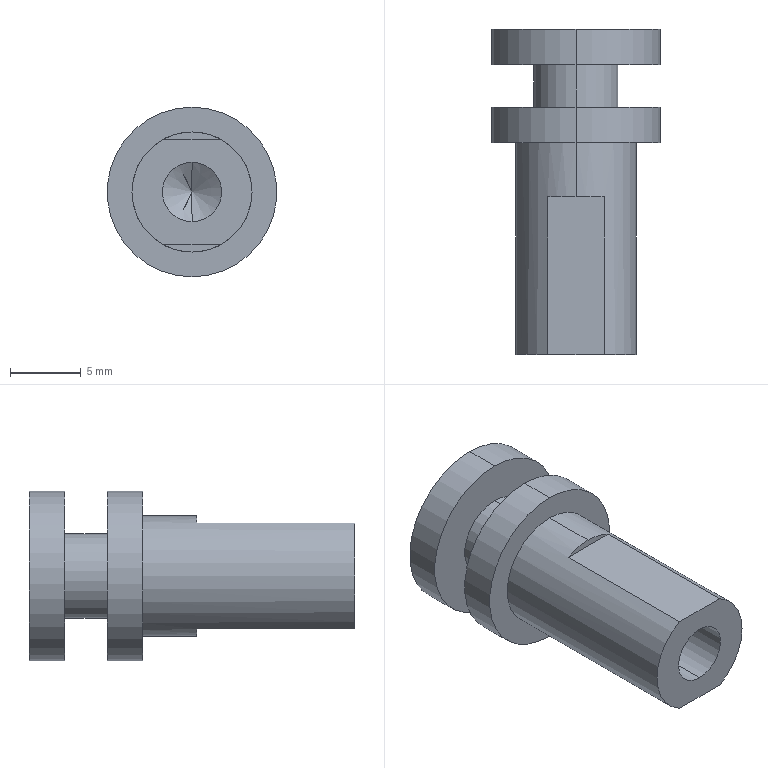Part | SolidWorks | features ICE 5, 3DProfileFeature 1, Extrusion 1, HoleWzd 1 | 1 solid | 21 faces | box 12 x 23 x 12 mm | volume 1299 mm3 | cylinder 10 | plane 9 | cone 2 | commonest cylinder face diameters 12 x4 4.2 x2 6 x2 8.5 x2
STEP:
#1=CARTESIAN_POINT('',(0.,-5.5,2.1));
#2=VERTEX_POINT('',#1);
#3=CARTESIAN_POINT('',(0.,-5.5,-2.1));
#4=VERTEX_POINT('',#3);
#5=CARTESIAN_POINT('',(0.,-5.5,0.));
#6=DIRECTION('',(0.,-1.,0.));
#7=DIRECTION('',(0.,0.,-1.));
#8=AXIS2_PLACEMENT_3D('',#5,#6,#7);
#9=CIRCLE('',#8,2.1);
#10=EDGE_CURVE('',#2,#4,#9,.T.);
#11=ORIENTED_EDGE('',*,*,#10,.F.);
#12=CARTESIAN_POINT('',(0.,-17.5,2.1));
#13=VERTEX_POINT('',#12);
#14=CARTESIAN_POINT('',(0.,-17.5,2.1));
#15=DIRECTION('',(0.,-1.,0.));
#16=VECTOR('',#15,1000.);
#17=LINE('',#14,#16);
#18=EDGE_CURVE('',#2,#13,#17,.T.);
#19=ORIENTED_EDGE('',*,*,#18,.T.);
#20=CARTESIAN_POINT('',(0.,-17.5,-2.1));
#21=VERTEX_POINT('',#20);
#22=CARTESIAN_POINT('',(0.,-17.5,0.));
#23=DIRECTION('',(0.,-1.,0.));
#24=DIRECTION('',(0.,0.,-1.));
#25=AXIS2_PLACEMENT_3D('',#22,#23,#24);
#26=CIRCLE('',#25,2.1);
#27=EDGE_CURVE('',#13,#21,#26,.T.);
#28=ORIENTED_EDGE('',*,*,#27,.T.);
#29=CARTESIAN_POINT('',(0.,-17.5,-2.1));
#30=DIRECTION('',(0.,-1.,0.));
#31=VECTOR('',#30,1000.);
#32=LINE('',#29,#31);
#33=EDGE_CURVE('',#4,#21,#32,.T.);
#34=ORIENTED_EDGE('',*,*,#33,.F.);
#35=EDGE_LOOP('',(#11,#19,#28,#34));
#36=FACE_OUTER_BOUND('',#35,.T.);
#37=CARTESIAN_POINT('',(0.,-17.5,0.));
#38=DIRECTION('',(0.,-1.,0.));
#39=DIRECTION('',(0.,0.,-1.));
#40=AXIS2_PLACEMENT_3D('',#37,#38,#39);
#41=CYLINDRICAL_SURFACE('',#40,2.1);
#42=ADVANCED_FACE('',(#36),#41,.F.);
#43=CARTESIAN_POINT('',(0.,-4.238,0.));
#44=VERTEX_POINT('',#43);
#45=CARTESIAN_POINT('',(0.,-5.5,-2.1));
#46=DIRECTION('',(0.,-0.515,-0.8572));
#47=VECTOR('',#46,1000.);
#48=LINE('',#45,#47);
#49=EDGE_CURVE('',#44,#4,#48,.T.);
#50=ORIENTED_EDGE('',*,*,#49,.F.);
#51=CARTESIAN_POINT('',(0.,-5.5,2.1));
#52=DIRECTION('',(0.,-0.515,0.8572));
#53=VECTOR('',#52,1000.);
#54=LINE('',#51,#53);
#55=EDGE_CURVE('',#44,#2,#54,.T.);
#56=ORIENTED_EDGE('',*,*,#55,.T.);
#57=ORIENTED_EDGE('',*,*,#10,.T.);
#58=EDGE_LOOP('',(#50,#56,#57));
#59=FACE_OUTER_BOUND('',#58,.T.);
#60=CARTESIAN_POINT('',(0.,-5.5,0.));
#61=DIRECTION('',(0.,-1.,0.));
#62=DIRECTION('',(0.,0.,-1.));
#63=AXIS2_PLACEMENT_3D('',#60,#61,#62);
#64=CONICAL_SURFACE('',#63,2.1,1.03);
#65=ADVANCED_FACE('',(#59),#64,.F.);
#66=CARTESIAN_POINT('',(2.,-6.347,-3.75));
#67=VERTEX_POINT('',#66);
#68=CARTESIAN_POINT('',(0.,-6.347,-4.25));
#69=VERTEX_POINT('',#68);
#70=CARTESIAN_POINT('',(0.,-6.347,0.));
#71=DIRECTION('',(0.,1.,0.));
#72=DIRECTION('',(0.,0.,1.));
#73=AXIS2_PLACEMENT_3D('',#70,#71,#72);
#74=CIRCLE('',#73,4.25);
#75=EDGE_CURVE('',#67,#69,#74,.T.);
#76=ORIENTED_EDGE('',*,*,#75,.T.);
#77=CARTESIAN_POINT('',(0.,-2.5,-4.25));
#78=VERTEX_POINT('',#77);
#79=CARTESIAN_POINT('',(0.,-17.5,-4.25));
#80=DIRECTION('',(0.,1.,0.));
#81=VECTOR('',#80,1000.);
#82=LINE('',#79,#81);
#83=EDGE_CURVE('',#69,#78,#82,.T.);
#84=ORIENTED_EDGE('',*,*,#83,.T.);
#85=CARTESIAN_POINT('',(0.,-2.5,4.25));
#86=VERTEX_POINT('',#85);
#87=CARTESIAN_POINT('',(0.,-2.5,0.));
#88=DIRECTION('',(0.,-1.,0.));
#89=DIRECTION('',(0.,0.,-1.));
#90=AXIS2_PLACEMENT_3D('',#87,#88,#89);
#91=CIRCLE('',#90,4.25);
#92=EDGE_CURVE('',#78,#86,#91,.T.);
#93=ORIENTED_EDGE('',*,*,#92,.T.);
#94=CARTESIAN_POINT('',(0.,-6.347,4.25));
#95=VERTEX_POINT('',#94);
#96=CARTESIAN_POINT('',(0.,-17.5,4.25));
#97=DIRECTION('',(0.,1.,0.));
#98=VECTOR('',#97,1000.);
#99=LINE('',#96,#98);
#100=EDGE_CURVE('',#95,#86,#99,.T.);
#101=ORIENTED_EDGE('',*,*,#100,.F.);
#102=CARTESIAN_POINT('',(2.,-6.347,3.75));
#103=VERTEX_POINT('',#102);
#104=CARTESIAN_POINT('',(0.,-6.347,0.));
#105=DIRECTION('',(0.,1.,0.));
#106=DIRECTION('',(0.,0.,1.));
#107=AXIS2_PLACEMENT_3D('',#104,#105,#106);
#108=CIRCLE('',#107,4.25);
#109=EDGE_CURVE('',#95,#103,#108,.T.);
#110=ORIENTED_EDGE('',*,*,#109,.T.);
#111=CARTESIAN_POINT('',(2.,-17.5,3.75));
#112=VERTEX_POINT('',#111);
#113=CARTESIAN_POINT('',(2.,-17.5,3.75));
#114=DIRECTION('',(0.,-1.,0.));
#115=VECTOR('',#114,1000.);
#116=LINE('',#113,#115);
#117=EDGE_CURVE('',#103,#112,#116,.T.);
#118=ORIENTED_EDGE('',*,*,#117,.T.);
#119=CARTESIAN_POINT('',(2.,-17.5,-3.75));
#120=VERTEX_POINT('',#119);
#121=CARTESIAN_POINT('',(0.,-17.5,0.));
#122=DIRECTION('',(0.,-1.,0.));
#123=DIRECTION('',(0.,0.,-1.));
#124=AXIS2_PLACEMENT_3D('',#121,#122,#123);
#125=CIRCLE('',#124,4.25);
#126=EDGE_CURVE('',#120,#112,#125,.T.);
#127=ORIENTED_EDGE('',*,*,#126,.F.);
#128=CARTESIAN_POINT('',(2.,-17.5,-3.75));
#129=DIRECTION('',(0.,1.,0.));
#130=VECTOR('',#129,1000.);
#131=LINE('',#128,#130);
#132=EDGE_CURVE('',#120,#67,#131,.T.);
#133=ORIENTED_EDGE('',*,*,#132,.T.);
#134=EDGE_LOOP('',(#76,#84,#93,#101,#110,#118,#127,#133));
#135=FACE_OUTER_BOUND('',#134,.T.);
#136=CARTESIAN_POINT('',(0.,-17.5,0.));
#137=DIRECTION('',(0.,1.,0.));
#138=DIRECTION('',(0.,0.,1.));
#139=AXIS2_PLACEMENT_3D('',#136,#137,#138);
#140=CYLINDRICAL_SURFACE('',#139,4.25);
#141=ADVANCED_FACE('',(#135),#140,.T.);
#142=CARTESIAN_POINT('',(0.,-2.5,-6.));
#143=VERTEX_POINT('',#142);
#144=CARTESIAN_POINT('',(0.,-2.5,6.));
#145=VERTEX_POINT('',#144);
#146=CARTESIAN_POINT('',(0.,-2.5,0.));
#147=DIRECTION('',(0.,-1.,0.));
#148=DIRECTION('',(0.,0.,-1.));
#149=AXIS2_PLACEMENT_3D('',#146,#147,#148);
#150=CIRCLE('',#149,6.);
#151=EDGE_CURVE('',#143,#145,#150,.T.);
#152=ORIENTED_EDGE('',*,*,#151,.F.);
#153=CARTESIAN_POINT('',(0.,0.,-6.));
#154=VERTEX_POINT('',#153);
#155=CARTESIAN_POINT('',(0.,-2.5,-6.));
#156=DIRECTION('',(0.,1.,0.));
#157=VECTOR('',#156,1000.);
#158=LINE('',#155,#157);
#159=EDGE_CURVE('',#143,#154,#158,.T.);
#160=ORIENTED_EDGE('',*,*,#159,.T.);
#161=CARTESIAN_POINT('',(0.,0.,6.));
#162=VERTEX_POINT('',#161);
#163=CARTESIAN_POINT('',(0.,0.,0.));
#164=DIRECTION('',(0.,-1.,0.));
#165=DIRECTION('',(0.,0.,-1.));
#166=AXIS2_PLACEMENT_3D('',#163,#164,#165);
#167=CIRCLE('',#166,6.);
#168=EDGE_CURVE('',#154,#162,#167,.T.);
#169=ORIENTED_EDGE('',*,*,#168,.T.);
#170=CARTESIAN_POINT('',(0.,-2.5,6.));
#171=DIRECTION('',(0.,1.,0.));
#172=VECTOR('',#171,1000.);
#173=LINE('',#170,#172);
#174=EDGE_CURVE('',#145,#162,#173,.T.);
#175=ORIENTED_EDGE('',*,*,#174,.F.);
#176=EDGE_LOOP('',(#152,#160,#169,#175));
#177=FACE_OUTER_BOUND('',#176,.T.);
#178=CARTESIAN_POINT('',(0.,-2.5,0.));
#179=DIRECTION('',(0.,1.,0.));
#180=DIRECTION('',(0.,0.,1.));
#181=AXIS2_PLACEMENT_3D('',#178,#179,#180);
#182=CYLINDRICAL_SURFACE('',#181,6.);
#183=ADVANCED_FACE('',(#177),#182,.T.);
#184=CARTESIAN_POINT('',(0.,5.5,6.));
#185=VERTEX_POINT('',#184);
#186=CARTESIAN_POINT('',(0.,5.5,-6.));
#187=VERTEX_POINT('',#186);
#188=CARTESIAN_POINT('',(0.,5.5,0.));
#189=DIRECTION('',(0.,1.,0.));
#190=DIRECTION('',(0.,0.,1.));
#191=AXIS2_PLACEMENT_3D('',#188,#189,#190);
#192=CIRCLE('',#191,6.);
#193=EDGE_CURVE('',#185,#187,#192,.T.);
#194=ORIENTED_EDGE('',*,*,#193,.F.);
#195=CARTESIAN_POINT('',(0.,3.,6.));
#196=VERTEX_POINT('',#195);
#197=CARTESIAN_POINT('',(0.,5.5,6.));
#198=DIRECTION('',(0.,-1.,0.));
#199=VECTOR('',#198,1000.);
#200=LINE('',#197,#199);
#201=EDGE_CURVE('',#185,#196,#200,.T.);
#202=ORIENTED_EDGE('',*,*,#201,.T.);
#203=CARTESIAN_POINT('',(0.,3.,-6.));
#204=VERTEX_POINT('',#203);
#205=CARTESIAN_POINT('',(0.,3.,0.));
#206=DIRECTION('',(0.,1.,0.));
#207=DIRECTION('',(0.,0.,1.));
#208=AXIS2_PLACEMENT_3D('',#205,#206,#207);
#209=CIRCLE('',#208,6.);
#210=EDGE_CURVE('',#196,#204,#209,.T.);
#211=ORIENTED_EDGE('',*,*,#210,.T.);
#212=CARTESIAN_POINT('',(0.,5.5,-6.));
#213=DIRECTION('',(0.,-1.,0.));
#214=VECTOR('',#213,1000.);
#215=LINE('',#212,#214);
#216=EDGE_CURVE('',#187,#204,#215,.T.);
#217=ORIENTED_EDGE('',*,*,#216,.F.);
#218=EDGE_LOOP('',(#194,#202,#211,#217));
#219=FACE_OUTER_BOUND('',#218,.T.);
#220=CARTESIAN_POINT('',(0.,5.5,0.));
#221=DIRECTION('',(0.,-1.,0.));
#222=DIRECTION('',(0.,0.,-1.));
#223=AXIS2_PLACEMENT_3D('',#220,#221,#222);
#224=CYLINDRICAL_SURFACE('',#223,6.);
#225=ADVANCED_FACE('',(#219),#224,.T.);
#226=CARTESIAN_POINT('',(0.,3.,3.));
#227=VERTEX_POINT('',#226);
#228=CARTESIAN_POINT('',(0.,3.,-3.));
#229=VERTEX_POINT('',#228);
#230=CARTESIAN_POINT('',(0.,3.,0.));
#231=DIRECTION('',(0.,1.,0.));
#232=DIRECTION('',(0.,0.,1.));
#233=AXIS2_PLACEMENT_3D('',#230,#231,#232);
#234=CIRCLE('',#233,3.);
#235=EDGE_CURVE('',#227,#229,#234,.T.);
#236=ORIENTED_EDGE('',*,*,#235,.F.);
#237=CARTESIAN_POINT('',(0.,0.,3.));
#238=VERTEX_POINT('',#237);
#239=CARTESIAN_POINT('',(0.,3.,3.));
#240=DIRECTION('',(0.,-1.,0.));
#241=VECTOR('',#240,1000.);
#242=LINE('',#239,#241);
#243=EDGE_CURVE('',#227,#238,#242,.T.);
#244=ORIENTED_EDGE('',*,*,#243,.T.);
#245=CARTESIAN_POINT('',(0.,0.,-3.));
#246=VERTEX_POINT('',#245);
#247=CARTESIAN_POINT('',(0.,0.,0.));
#248=DIRECTION('',(0.,-1.,0.));
#249=DIRECTION('',(0.,0.,-1.));
#250=AXIS2_PLACEMENT_3D('',#247,#248,#249);
#251=CIRCLE('',#250,3.);
#252=EDGE_CURVE('',#246,#238,#251,.T.);
#253=ORIENTED_EDGE('',*,*,#252,.F.);
#254=CARTESIAN_POINT('',(0.,3.,-3.));
#255=DIRECTION('',(0.,-1.,0.));
#256=VECTOR('',#255,1000.);
#257=LINE('',#254,#256);
#258=EDGE_CURVE('',#229,#246,#257,.T.);
#259=ORIENTED_EDGE('',*,*,#258,.F.);
#260=EDGE_LOOP('',(#236,#244,#253,#259));
#261=FACE_OUTER_BOUND('',#260,.T.);
#262=CARTESIAN_POINT('',(0.,3.,0.));
#263=DIRECTION('',(0.,-1.,0.));
#264=DIRECTION('',(0.,0.,-1.));
#265=AXIS2_PLACEMENT_3D('',#262,#263,#264);
#266=CYLINDRICAL_SURFACE('',#265,3.);
#267=ADVANCED_FACE('',(#261),#266,.T.);
#268=CARTESIAN_POINT('',(0.,-2.5,0.));
#269=DIRECTION('',(0.,-1.,0.));
#270=DIRECTION('',(0.,0.,-1.));
#271=AXIS2_PLACEMENT_3D('',#268,#269,#270);
#272=CIRCLE('',#271,6.);
#273=EDGE_CURVE('',#145,#143,#272,.T.);
#274=ORIENTED_EDGE('',*,*,#273,.T.);
#275=ORIENTED_EDGE('',*,*,#151,.T.);
#276=EDGE_LOOP('',(#274,#275));
#277=FACE_OUTER_BOUND('',#276,.T.);
#278=CARTESIAN_POINT('',(0.,-2.5,0.));
#279=DIRECTION('',(0.,-1.,0.));
#280=DIRECTION('',(0.,0.,-1.));
#281=AXIS2_PLACEMENT_3D('',#278,#279,#280);
#282=CIRCLE('',#281,4.25);
#283=EDGE_CURVE('',#86,#78,#282,.T.);
#284=ORIENTED_EDGE('',*,*,#283,.F.);
#285=ORIENTED_EDGE('',*,*,#92,.F.);
#286=EDGE_LOOP('',(#284,#285));
#287=FACE_BOUND('',#286,.T.);
#288=CARTESIAN_POINT('',(0.,-2.5,0.));
#289=DIRECTION('',(0.,-1.,0.));
#290=DIRECTION('',(0.,0.,-1.));
#291=AXIS2_PLACEMENT_3D('',#288,#289,#290);
#292=PLANE('',#291);
#293=ADVANCED_FACE('',(#277,#287),#292,.T.);
#294=ORIENTED_EDGE('',*,*,#243,.F.);
#295=CARTESIAN_POINT('',(0.,3.,0.));
#296=DIRECTION('',(0.,1.,0.));
#297=DIRECTION('',(0.,0.,1.));
#298=AXIS2_PLACEMENT_3D('',#295,#296,#297);
#299=CIRCLE('',#298,3.);
#300=EDGE_CURVE('',#229,#227,#299,.T.);
#301=ORIENTED_EDGE('',*,*,#300,.F.);
#302=ORIENTED_EDGE('',*,*,#258,.T.);
#303=CARTESIAN_POINT('',(0.,0.,0.));
#304=DIRECTION('',(0.,-1.,0.));
#305=DIRECTION('',(0.,0.,-1.));
#306=AXIS2_PLACEMENT_3D('',#303,#304,#305);
#307=CIRCLE('',#306,3.);
#308=EDGE_CURVE('',#238,#246,#307,.T.);
#309=ORIENTED_EDGE('',*,*,#308,.F.);
#310=EDGE_LOOP('',(#294,#301,#302,#309));
#311=FACE_OUTER_BOUND('',#310,.T.);
#312=CARTESIAN_POINT('',(0.,3.,0.));
#313=DIRECTION('',(0.,-1.,0.));
#314=DIRECTION('',(0.,0.,-1.));
#315=AXIS2_PLACEMENT_3D('',#312,#313,#314);
#316=CYLINDRICAL_SURFACE('',#315,3.);
#317=ADVANCED_FACE('',(#311),#316,.T.);
#318=CARTESIAN_POINT('',(0.,3.,0.));
#319=DIRECTION('',(0.,1.,0.));
#320=DIRECTION('',(0.,0.,1.));
#321=AXIS2_PLACEMENT_3D('',#318,#319,#320);
#322=CIRCLE('',#321,6.);
#323=EDGE_CURVE('',#204,#196,#322,.T.);
#324=ORIENTED_EDGE('',*,*,#323,.F.);
#325=ORIENTED_EDGE('',*,*,#210,.F.);
#326=EDGE_LOOP('',(#324,#325));
#327=FACE_OUTER_BOUND('',#326,.T.);
#328=ORIENTED_EDGE('',*,*,#300,.T.);
#329=ORIENTED_EDGE('',*,*,#235,.T.);
#330=EDGE_LOOP('',(#328,#329));
#331=FACE_BOUND('',#330,.T.);
#332=CARTESIAN_POINT('',(0.,3.,0.));
#333=DIRECTION('',(0.,1.,0.));
#334=DIRECTION('',(0.,0.,1.));
#335=AXIS2_PLACEMENT_3D('',#332,#333,#334);
#336=PLANE('',#335);
#337=ADVANCED_FACE('',(#327,#331),#336,.F.);
#338=ORIENTED_EDGE('',*,*,#201,.F.);
#339=CARTESIAN_POINT('',(0.,5.5,0.));
#340=DIRECTION('',(0.,1.,0.));
#341=DIRECTION('',(0.,0.,1.));
#342=AXIS2_PLACEMENT_3D('',#339,#340,#341);
#343=CIRCLE('',#342,6.);
#344=EDGE_CURVE('',#187,#185,#343,.T.);
#345=ORIENTED_EDGE('',*,*,#344,.F.);
#346=ORIENTED_EDGE('',*,*,#216,.T.);
#347=ORIENTED_EDGE('',*,*,#323,.T.);
#348=EDGE_LOOP('',(#338,#345,#346,#347));
#349=FACE_OUTER_BOUND('',#348,.T.);
#350=CARTESIAN_POINT('',(0.,5.5,0.));
#351=DIRECTION('',(0.,-1.,0.));
#352=DIRECTION('',(0.,0.,-1.));
#353=AXIS2_PLACEMENT_3D('',#350,#351,#352);
#354=CYLINDRICAL_SURFACE('',#353,6.);
#355=ADVANCED_FACE('',(#349),#354,.T.);
#356=ORIENTED_EDGE('',*,*,#344,.T.);
#357=ORIENTED_EDGE('',*,*,#193,.T.);
#358=EDGE_LOOP('',(#356,#357));
#359=FACE_OUTER_BOUND('',#358,.T.);
#360=CARTESIAN_POINT('',(0.,5.5,0.));
#361=DIRECTION('',(0.,1.,0.));
#362=DIRECTION('',(0.,0.,1.));
#363=AXIS2_PLACEMENT_3D('',#360,#361,#362);
#364=PLANE('',#363);
#365=ADVANCED_FACE('',(#359),#364,.T.);
#366=CARTESIAN_POINT('',(0.,0.,0.));
#367=DIRECTION('',(0.,-1.,0.));
#368=DIRECTION('',(0.,0.,-1.));
#369=AXIS2_PLACEMENT_3D('',#366,#367,#368);
#370=CIRCLE('',#369,6.);
#371=EDGE_CURVE('',#162,#154,#370,.T.);
#372=ORIENTED_EDGE('',*,*,#371,.F.);
#373=ORIENTED_EDGE('',*,*,#168,.F.);
#374=EDGE_LOOP('',(#372,#373));
#375=FACE_OUTER_BOUND('',#374,.T.);
#376=ORIENTED_EDGE('',*,*,#252,.T.);
#377=ORIENTED_EDGE('',*,*,#308,.T.);
#378=EDGE_LOOP('',(#376,#377));
#379=FACE_BOUND('',#378,.T.);
#380=CARTESIAN_POINT('',(0.,0.,0.));
#381=DIRECTION('',(0.,-1.,0.));
#382=DIRECTION('',(0.,0.,-1.));
#383=AXIS2_PLACEMENT_3D('',#380,#381,#382);
#384=PLANE('',#383);
#385=ADVANCED_FACE('',(#375,#379),#384,.F.);
#386=ORIENTED_EDGE('',*,*,#159,.F.);
#387=ORIENTED_EDGE('',*,*,#273,.F.);
#388=ORIENTED_EDGE('',*,*,#174,.T.);
#389=ORIENTED_EDGE('',*,*,#371,.T.);
#390=EDGE_LOOP('',(#386,#387,#388,#389));
#391=FACE_OUTER_BOUND('',#390,.T.);
#392=CARTESIAN_POINT('',(0.,-2.5,0.));
#393=DIRECTION('',(0.,1.,0.));
#394=DIRECTION('',(0.,0.,1.));
#395=AXIS2_PLACEMENT_3D('',#392,#393,#394);
#396=CYLINDRICAL_SURFACE('',#395,6.);
#397=ADVANCED_FACE('',(#391),#396,.T.);
#398=ORIENTED_EDGE('',*,*,#83,.F.);
#399=CARTESIAN_POINT('',(-2.,-6.347,-3.75));
#400=VERTEX_POINT('',#399);
#401=CARTESIAN_POINT('',(0.,-6.347,0.));
#402=DIRECTION('',(0.,1.,0.));
#403=DIRECTION('',(0.,0.,1.));
#404=AXIS2_PLACEMENT_3D('',#401,#402,#403);
#405=CIRCLE('',#404,4.25);
#406=EDGE_CURVE('',#69,#400,#405,.T.);
#407=ORIENTED_EDGE('',*,*,#406,.T.);
#408=CARTESIAN_POINT('',(-2.,-17.5,-3.75));
#409=VERTEX_POINT('',#408);
#410=CARTESIAN_POINT('',(-2.,-17.5,-3.75));
#411=DIRECTION('',(0.,-1.,0.));
#412=VECTOR('',#411,1000.);
#413=LINE('',#410,#412);
#414=EDGE_CURVE('',#400,#409,#413,.T.);
#415=ORIENTED_EDGE('',*,*,#414,.T.);
#416=CARTESIAN_POINT('',(-2.,-17.5,3.75));
#417=VERTEX_POINT('',#416);
#418=CARTESIAN_POINT('',(0.,-17.5,0.));
#419=DIRECTION('',(0.,-1.,0.));
#420=DIRECTION('',(0.,0.,-1.));
#421=AXIS2_PLACEMENT_3D('',#418,#419,#420);
#422=CIRCLE('',#421,4.25);
#423=EDGE_CURVE('',#417,#409,#422,.T.);
#424=ORIENTED_EDGE('',*,*,#423,.F.);
#425=CARTESIAN_POINT('',(-2.,-6.347,3.75));
#426=VERTEX_POINT('',#425);
#427=CARTESIAN_POINT('',(-2.,-17.5,3.75));
#428=DIRECTION('',(0.,1.,0.));
#429=VECTOR('',#428,1000.);
#430=LINE('',#427,#429);
#431=EDGE_CURVE('',#417,#426,#430,.T.);
#432=ORIENTED_EDGE('',*,*,#431,.T.);
#433=CARTESIAN_POINT('',(0.,-6.347,0.));
#434=DIRECTION('',(0.,1.,0.));
#435=DIRECTION('',(0.,0.,1.));
#436=AXIS2_PLACEMENT_3D('',#433,#434,#435);
#437=CIRCLE('',#436,4.25);
#438=EDGE_CURVE('',#426,#95,#437,.T.);
#439=ORIENTED_EDGE('',*,*,#438,.T.);
#440=ORIENTED_EDGE('',*,*,#100,.T.);
#441=ORIENTED_EDGE('',*,*,#283,.T.);
#442=EDGE_LOOP('',(#398,#407,#415,#424,#432,#439,#440,#441));
#443=FACE_OUTER_BOUND('',#442,.T.);
#444=CARTESIAN_POINT('',(0.,-17.5,0.));
#445=DIRECTION('',(0.,1.,0.));
#446=DIRECTION('',(0.,0.,1.));
#447=AXIS2_PLACEMENT_3D('',#444,#445,#446);
#448=CYLINDRICAL_SURFACE('',#447,4.25);
#449=ADVANCED_FACE('',(#443),#448,.T.);
#450=CARTESIAN_POINT('',(0.,-17.5,3.75));
#451=DIRECTION('',(1.,0.,0.));
#452=VECTOR('',#451,1000.);
#453=LINE('',#450,#452);
#454=EDGE_CURVE('',#417,#112,#453,.T.);
#455=ORIENTED_EDGE('',*,*,#454,.F.);
#456=ORIENTED_EDGE('',*,*,#423,.T.);
#457=CARTESIAN_POINT('',(0.,-17.5,-3.75));
#458=DIRECTION('',(-1.,0.,0.));
#459=VECTOR('',#458,1000.);
#460=LINE('',#457,#459);
#461=EDGE_CURVE('',#120,#409,#460,.T.);
#462=ORIENTED_EDGE('',*,*,#461,.F.);
#463=ORIENTED_EDGE('',*,*,#126,.T.);
#464=EDGE_LOOP('',(#455,#456,#462,#463));
#465=FACE_OUTER_BOUND('',#464,.T.);
#466=CARTESIAN_POINT('',(0.,-17.5,0.));
#467=DIRECTION('',(0.,-1.,0.));
#468=DIRECTION('',(0.,0.,-1.));
#469=AXIS2_PLACEMENT_3D('',#466,#467,#468);
#470=CIRCLE('',#469,2.1);
#471=EDGE_CURVE('',#21,#13,#470,.T.);
#472=ORIENTED_EDGE('',*,*,#471,.F.);
#473=ORIENTED_EDGE('',*,*,#27,.F.);
#474=EDGE_LOOP('',(#472,#473));
#475=FACE_BOUND('',#474,.T.);
#476=CARTESIAN_POINT('',(0.,-17.5,0.));
#477=DIRECTION('',(0.,-1.,0.));
#478=DIRECTION('',(0.,0.,-1.));
#479=AXIS2_PLACEMENT_3D('',#476,#477,#478);
#480=PLANE('',#479);
#481=ADVANCED_FACE('',(#465,#475),#480,.T.);
#482=ORIENTED_EDGE('',*,*,#55,.F.);
#483=ORIENTED_EDGE('',*,*,#49,.T.);
#484=CARTESIAN_POINT('',(0.,-5.5,0.));
#485=DIRECTION('',(0.,-1.,0.));
#486=DIRECTION('',(0.,0.,-1.));
#487=AXIS2_PLACEMENT_3D('',#484,#485,#486);
#488=CIRCLE('',#487,2.1);
#489=EDGE_CURVE('',#4,#2,#488,.T.);
#490=ORIENTED_EDGE('',*,*,#489,.T.);
#491=EDGE_LOOP('',(#482,#483,#490));
#492=FACE_OUTER_BOUND('',#491,.T.);
#493=CARTESIAN_POINT('',(0.,-5.5,0.));
#494=DIRECTION('',(0.,-1.,0.));
#495=DIRECTION('',(0.,0.,-1.));
#496=AXIS2_PLACEMENT_3D('',#493,#494,#495);
#497=CONICAL_SURFACE('',#496,2.1,1.03);
#498=ADVANCED_FACE('',(#492),#497,.F.);
#499=ORIENTED_EDGE('',*,*,#18,.F.);
#500=ORIENTED_EDGE('',*,*,#489,.F.);
#501=ORIENTED_EDGE('',*,*,#33,.T.);
#502=ORIENTED_EDGE('',*,*,#471,.T.);
#503=EDGE_LOOP('',(#499,#500,#501,#502));
#504=FACE_OUTER_BOUND('',#503,.T.);
#505=CARTESIAN_POINT('',(0.,-17.5,0.));
#506=DIRECTION('',(0.,-1.,0.));
#507=DIRECTION('',(0.,0.,-1.));
#508=AXIS2_PLACEMENT_3D('',#505,#506,#507);
#509=CYLINDRICAL_SURFACE('',#508,2.1);
#510=ADVANCED_FACE('',(#504),#509,.F.);
#511=CARTESIAN_POINT('',(-5.,-6.347,-3.75));
#512=DIRECTION('',(1.,0.,0.));
#513=VECTOR('',#512,1000.);
#514=LINE('',#511,#513);
#515=EDGE_CURVE('',#400,#67,#514,.T.);
#516=ORIENTED_EDGE('',*,*,#515,.F.);
#517=ORIENTED_EDGE('',*,*,#406,.F.);
#518=ORIENTED_EDGE('',*,*,#75,.F.);
#519=EDGE_LOOP('',(#516,#517,#518));
#520=FACE_OUTER_BOUND('',#519,.T.);
#521=CARTESIAN_POINT('',(-5.,-6.347,-3.75));
#522=DIRECTION('',(0.,1.,0.));
#523=DIRECTION('',(0.,0.,1.));
#524=AXIS2_PLACEMENT_3D('',#521,#522,#523);
#525=PLANE('',#524);
#526=ADVANCED_FACE('',(#520),#525,.F.);
#527=ORIENTED_EDGE('',*,*,#461,.T.);
#528=ORIENTED_EDGE('',*,*,#414,.F.);
#529=ORIENTED_EDGE('',*,*,#515,.T.);
#530=ORIENTED_EDGE('',*,*,#132,.F.);
#531=EDGE_LOOP('',(#527,#528,#529,#530));
#532=FACE_OUTER_BOUND('',#531,.T.);
#533=CARTESIAN_POINT('',(-5.,-17.5,-3.75));
#534=DIRECTION('',(0.,0.,1.));
#535=DIRECTION('',(1.,0.,0.));
#536=AXIS2_PLACEMENT_3D('',#533,#534,#535);
#537=PLANE('',#536);
#538=ADVANCED_FACE('',(#532),#537,.F.);
#539=CARTESIAN_POINT('',(-5.,-6.347,3.75));
#540=DIRECTION('',(1.,0.,0.));
#541=VECTOR('',#540,1000.);
#542=LINE('',#539,#541);
#543=EDGE_CURVE('',#426,#103,#542,.T.);
#544=ORIENTED_EDGE('',*,*,#543,.T.);
#545=ORIENTED_EDGE('',*,*,#109,.F.);
#546=ORIENTED_EDGE('',*,*,#438,.F.);
#547=EDGE_LOOP('',(#544,#545,#546));
#548=FACE_OUTER_BOUND('',#547,.T.);
#549=CARTESIAN_POINT('',(-5.,-6.347,3.75));
#550=DIRECTION('',(0.,1.,0.));
#551=DIRECTION('',(0.,0.,1.));
#552=AXIS2_PLACEMENT_3D('',#549,#550,#551);
#553=PLANE('',#552);
#554=ADVANCED_FACE('',(#548),#553,.F.);
#555=ORIENTED_EDGE('',*,*,#454,.T.);
#556=ORIENTED_EDGE('',*,*,#117,.F.);
#557=ORIENTED_EDGE('',*,*,#543,.F.);
#558=ORIENTED_EDGE('',*,*,#431,.F.);
#559=EDGE_LOOP('',(#555,#556,#557,#558));
#560=FACE_OUTER_BOUND('',#559,.T.);
#561=CARTESIAN_POINT('',(-5.,-17.5,3.75));
#562=DIRECTION('',(0.,0.,-1.));
#563=DIRECTION('',(0.,1.,0.));
#564=AXIS2_PLACEMENT_3D('',#561,#562,#563);
#565=PLANE('',#564);
#566=ADVANCED_FACE('',(#560),#565,.F.);
#567=CLOSED_SHELL('',(#42,#65,#141,#183,#225,#267,#293,#317,#337,#355,#365,#385,#397,#449,#481,#498,#510,#526,#538,#554,#566));
#568=MANIFOLD_SOLID_BREP('',#567);
#569=CARTESIAN_POINT('',(0.,0.,0.));
#570=DIRECTION('',(0.,0.,1.));
#571=DIRECTION('',(1.,0.,0.));
#572=AXIS2_PLACEMENT_3D('',#569,#570,#571);
#573=(LENGTH_UNIT()NAMED_UNIT(*)SI_UNIT(.MILLI.,.METRE.));
#574=UNCERTAINTY_MEASURE_WITH_UNIT(LENGTH_MEASURE(0.00001),#573,'','');
#575=(NAMED_UNIT(*)PLANE_ANGLE_UNIT()SI_UNIT($,.RADIAN.));
#576=(NAMED_UNIT(*)SI_UNIT($,.STERADIAN.)SOLID_ANGLE_UNIT());
#577=(GEOMETRIC_REPRESENTATION_CONTEXT(3)GLOBAL_UNCERTAINTY_ASSIGNED_CONTEXT((#574))GLOBAL_UNIT_ASSIGNED_CONTEXT((#573,#575,#576))REPRESENTATION_CONTEXT('',''));
#578=ADVANCED_BREP_SHAPE_REPRESENTATION('',(#568,#572),#577);